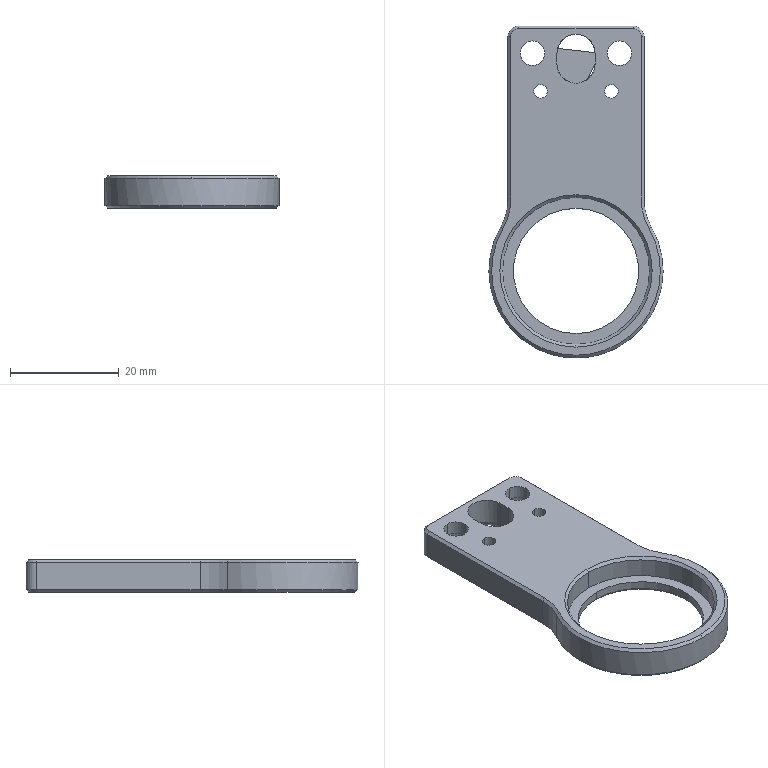NC program | NX | posted with a generic post | part box 32 x 61 x 6 mm
Lines 12416 to 12533 of 12533:
(PLANAR_PROFILE_COPY , TOOL : D6A45)
N24806 T01 M6
N24808 G54
N24810 G17 G0 G90 X-12.045 Y-6.8 S9500 M3
N24812 G43 Z30. H1
N24814 Z0.5
N24816 G94 G1 X-11.863 Z0.451 F500.
N24818 X-11.7 Y-6.637 Z0.389
N24820 Y-6.363 Z0.316
N24822 X-11.863 Y-6.2 Z0.254
N24824 X-12.137 Z0.181
N24826 X-12.3 Y-6.363 Z0.119
N24828 Y-6.637 Z0.045
N24830 X-12.137 Y-6.8 Z-0.016
N24832 X-11.863 Z-0.09
N24834 X-11.7 Y-6.637 Z-0.152
N24836 Y-6.363 Z-0.225
N24838 X-11.863 Y-6.2 Z-0.287
N24840 X-12.137 Z-0.361
N24842 X-12.3 Y-6.363 Z-0.422
N24844 Y-6.637 Z-0.496
N24846 X-12.137 Y-6.8 Z-0.557
N24848 X-11.863 Z-0.631
N24850 X-11.7 Y-6.637 Z-0.693
N24852 Y-6.363 Z-0.766
N24854 X-11.863 Y-6.2 Z-0.828
N24856 X-12.137 Z-0.902
N24858 X-12.3 Y-6.363 Z-0.963
N24860 Y-6.5 Z-1.
N24862 G3 X-12. Y-6.8 R0.3 F1500.
N24864 X-12.3 Y-6.5 R-0.3
N24866 X-12.15 Y-6.76 R0.3
N24868 G1 Z0.5
N24870 G0 Z30.
N24872 X-4.651 Y-6.49
N24874 Z0.5
N24876 G1 Z-1. F500.
N24878 X-4.48 Y-5.75
N24880 G3 X-5. Y-5.45 R0.6
N24882 X-7.55 Y-8. R2.55 F1500.
N24884 X-5. Y-5.45 R-2.55
N24886 X-5.52 Y-5.75 R0.6
N24888 G1 X-5.349 Y-6.49
N24890 Z0.5
N24892 G0 Z30.
N24894 X-6.51 Y8.349
N24896 Z0.5
N24898 G1 Z-1. F500.
N24900 X-7.25 Y8.52
N24902 G3 X-7.55 Y8. R0.6
N24904 X-5. Y5.45 R2.55 F1500.
N24906 X-7.55 Y8. R-2.55
N24908 X-7.25 Y7.48 R0.6
N24910 G1 X-6.51 Y7.651
N24912 Z0.5
N24914 G0 Z30.
N24916 X-12.045 Y6.2
N24918 Z0.5
N24920 G1 X-11.863 Z0.451 F500.
N24922 X-11.7 Y6.363 Z0.389
N24924 Y6.637 Z0.316
N24926 X-11.863 Y6.8 Z0.254
N24928 X-12.137 Z0.181
N24930 X-12.3 Y6.637 Z0.119
N24932 Y6.363 Z0.045
N24934 X-12.137 Y6.2 Z-0.016
N24936 X-11.863 Z-0.09
N24938 X-11.7 Y6.363 Z-0.152
N24940 Y6.637 Z-0.225
N24942 X-11.863 Y6.8 Z-0.287
N24944 X-12.137 Z-0.361
N24946 X-12.3 Y6.637 Z-0.422
N24948 Y6.363 Z-0.496
N24950 X-12.137 Y6.2 Z-0.557
N24952 X-11.863 Z-0.631
N24954 X-11.7 Y6.363 Z-0.693
N24956 Y6.637 Z-0.766
N24958 X-11.863 Y6.8 Z-0.828
N24960 X-12.137 Z-0.902
N24962 X-12.3 Y6.637 Z-0.963
N24964 Y6.5 Z-1.
N24966 G3 X-12. Y6.2 R0.3 F1500.
N24968 X-12.3 Y6.5 R-0.3
N24970 X-12.15 Y6.24 R0.3
N24972 G1 Z0.5
N24974 G0 Z30.
N24976 X-35.403 Y-14.669
N24978 Z0.5
N24980 G1 Z-1. F500.
N24982 X-36.157 Y-14.235
N24984 G3 X-36.757 Y-14.236 R0.6
N24986 G2 X-36.757 Y14.236 R-16.45 F1500.
N24988 G3 X-31.971 Y12.95 R9.55
N24990 G1 X-2.
N24992 G2 X0.45 Y10.5 R2.45
N24994 G1 Y-10.5
N24996 G2 X-2. Y-12.95 R2.45
N24998 G1 X-31.971
N25000 G3 X-36.757 Y-14.236 R9.55
N25002 X-37.056 Y-14.756 R0.6
N25004 G1 X-37.055 Y-15.536
N25006 Z0.5
N25008 G0 Z30.
N25010 X-55.005 Y0.95
N25012 Z0.5
N25014 G1 Z-1. F500.
N25016 X-55.75 Y0.52
N25018 G3 X-56.05 Y0. R0.6
N25020 X-45. Y-11.05 R11.05 F1500.
N25022 X-56.05 Y0. R-11.05
N25024 X-55.75 Y-0.52 R0.6
N25026 G1 X-55.005 Y-0.95
N25028 Z0.5
N25030 G0 Z30.
N25032 M5
N25034 M2